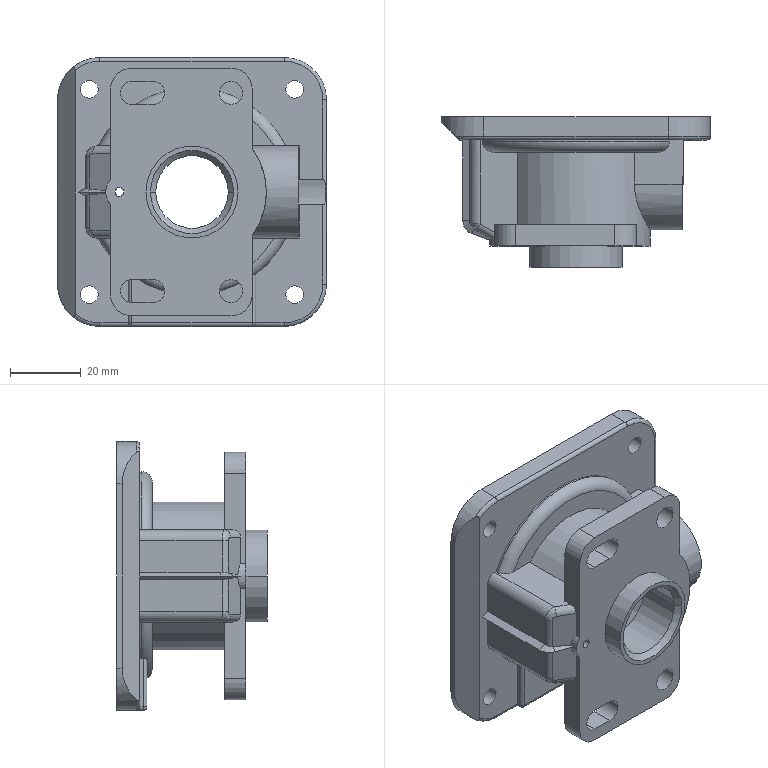Part | SolidWorks | features BaseBody 1 | 1 solid | 132 faces | box 76 x 42.5 x 76 mm | volume 52114 mm3 | cylinder 65 | plane 51 | cone 6 | torus 6 | sphere 2 | spline 2 | commonest cylinder face diameters 6.5 x10 2 x9 5 x8 4 x4 12 x4 24 x4